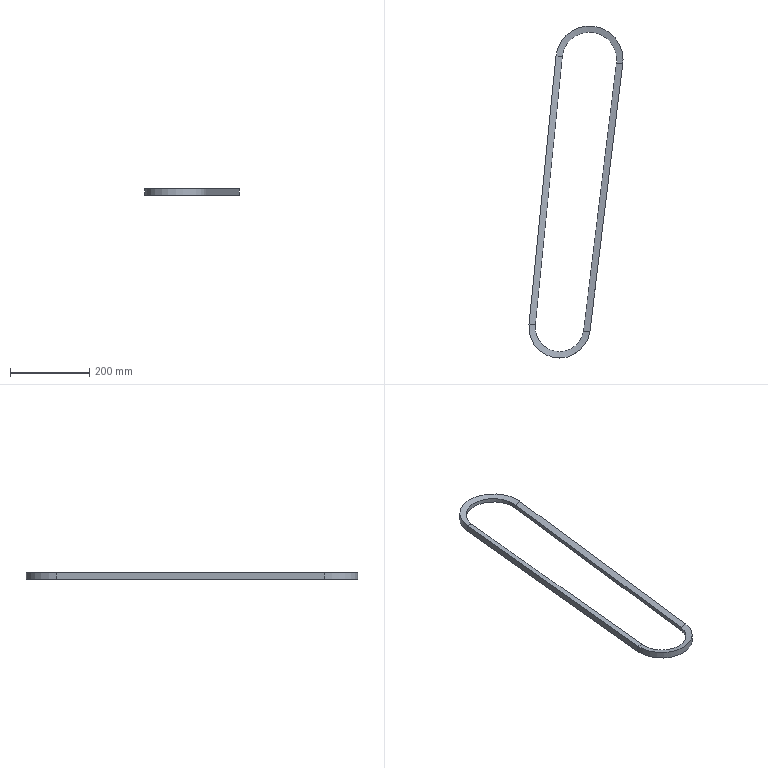Part | SolidWorks | features Sweep 1 | 1 solid | 18 faces | box 238 x 839.181 x 17 mm | volume 391508 mm3 | plane 8 | cylinder 6 | spline 4 | commonest cylinder face diameters 138.293 x2 170 x2 123.3 x1 155 x1
STEP:
#1=CARTESIAN_POINT('',(118.715,333.323,-5.));
#2=VERTEX_POINT('',#1);
#3=CARTESIAN_POINT('',(-19.01,342.17,-5.));
#4=VERTEX_POINT('',#3);
#5=CARTESIAN_POINT('',(49.568,333.323,-5.));
#6=DIRECTION('',(0.,0.,1.));
#7=DIRECTION('',(0.9887,-0.1498,0.));
#8=AXIS2_PLACEMENT_3D('',#5,#6,#7);
#9=CIRCLE('',#8,69.147);
#10=EDGE_CURVE('',#2,#4,#9,.T.);
#11=ORIENTED_EDGE('',*,*,#10,.F.);
#12=CARTESIAN_POINT('',(118.715,333.323,5.));
#13=VERTEX_POINT('',#12);
#14=CARTESIAN_POINT('',(118.715,333.323,0.));
#15=DIRECTION('',(0.,0.,1.));
#16=VECTOR('',#15,1000.);
#17=LINE('',#14,#16);
#18=EDGE_CURVE('',#2,#13,#17,.T.);
#19=ORIENTED_EDGE('',*,*,#18,.T.);
#20=CARTESIAN_POINT('',(-19.01,342.17,5.));
#21=VERTEX_POINT('',#20);
#22=CARTESIAN_POINT('',(49.568,333.323,5.));
#23=DIRECTION('',(0.,0.,1.));
#24=DIRECTION('',(0.9887,-0.1498,0.));
#25=AXIS2_PLACEMENT_3D('',#22,#23,#24);
#26=CIRCLE('',#25,69.147);
#27=EDGE_CURVE('',#13,#21,#26,.T.);
#28=ORIENTED_EDGE('',*,*,#27,.T.);
#29=CARTESIAN_POINT('',(-19.01,342.17,5.));
#30=DIRECTION('',(0.,0.,1.));
#31=VECTOR('',#30,1000.);
#32=LINE('',#29,#31);
#33=EDGE_CURVE('',#4,#21,#32,.T.);
#34=ORIENTED_EDGE('',*,*,#33,.F.);
#35=EDGE_LOOP('',(#11,#19,#28,#34));
#36=FACE_OUTER_BOUND('',#35,.T.);
#37=CARTESIAN_POINT('',(49.568,333.323,0.));
#38=DIRECTION('',(0.,0.,1.));
#39=DIRECTION('',(1.,0.,0.));
#40=AXIS2_PLACEMENT_3D('',#37,#38,#39);
#41=CYLINDRICAL_SURFACE('',#40,69.147);
#42=ADVANCED_FACE('',(#36),#41,.F.);
#43=CARTESIAN_POINT('',(133.935,322.968,-8.5));
#44=VERTEX_POINT('',#43);
#45=CARTESIAN_POINT('',(134.568,333.323,-8.5));
#46=VERTEX_POINT('',#45);
#47=CARTESIAN_POINT('',(49.568,333.323,-8.5));
#48=DIRECTION('',(0.,0.,1.));
#49=DIRECTION('',(0.9926,-0.1218,0.));
#50=AXIS2_PLACEMENT_3D('',#47,#48,#49);
#51=CIRCLE('',#50,85.);
#52=EDGE_CURVE('',#44,#46,#51,.T.);
#53=ORIENTED_EDGE('',*,*,#52,.T.);
#54=CARTESIAN_POINT('',(134.568,333.323,8.5));
#55=VERTEX_POINT('',#54);
#56=CARTESIAN_POINT('',(134.568,333.323,0.));
#57=DIRECTION('',(0.,0.,1.));
#58=VECTOR('',#57,1000.);
#59=LINE('',#56,#58);
#60=EDGE_CURVE('',#46,#55,#59,.T.);
#61=ORIENTED_EDGE('',*,*,#60,.T.);
#62=CARTESIAN_POINT('',(133.935,322.968,8.5));
#63=VERTEX_POINT('',#62);
#64=CARTESIAN_POINT('',(49.568,333.323,8.5));
#65=DIRECTION('',(0.,0.,1.));
#66=DIRECTION('',(0.9926,-0.1218,0.));
#67=AXIS2_PLACEMENT_3D('',#64,#65,#66);
#68=CIRCLE('',#67,85.);
#69=EDGE_CURVE('',#63,#55,#68,.T.);
#70=ORIENTED_EDGE('',*,*,#69,.F.);
#71=CARTESIAN_POINT('',(133.935,322.968,-8.5));
#72=DIRECTION('',(0.,0.,-1.));
#73=VECTOR('',#72,1000.);
#74=LINE('',#71,#73);
#75=EDGE_CURVE('',#63,#44,#74,.T.);
#76=ORIENTED_EDGE('',*,*,#75,.T.);
#77=EDGE_LOOP('',(#53,#61,#70,#76));
#78=FACE_OUTER_BOUND('',#77,.T.);
#79=CARTESIAN_POINT('',(49.568,333.323,0.));
#80=DIRECTION('',(0.,0.,1.));
#81=DIRECTION('',(1.,0.,0.));
#82=AXIS2_PLACEMENT_3D('',#79,#80,#81);
#83=CYLINDRICAL_SURFACE('',#82,85.);
#84=ADVANCED_FACE('',(#78),#83,.T.);
#85=CARTESIAN_POINT('',(50.991,-352.799,8.5));
#86=VERTEX_POINT('',#85);
#87=CARTESIAN_POINT('',(50.991,-352.799,8.5));
#88=DIRECTION('',(0.1218,0.9926,0.));
#89=VECTOR('',#88,1000.);
#90=LINE('',#87,#89);
#91=EDGE_CURVE('',#86,#63,#90,.T.);
#92=ORIENTED_EDGE('',*,*,#91,.F.);
#93=CARTESIAN_POINT('',(50.991,-352.799,-8.5));
#94=VERTEX_POINT('',#93);
#95=CARTESIAN_POINT('',(50.991,-352.799,-8.5));
#96=DIRECTION('',(0.,0.,-1.));
#97=VECTOR('',#96,1000.);
#98=LINE('',#95,#97);
#99=EDGE_CURVE('',#86,#94,#98,.T.);
#100=ORIENTED_EDGE('',*,*,#99,.T.);
#101=CARTESIAN_POINT('',(50.991,-352.799,-8.5));
#102=DIRECTION('',(0.1218,0.9926,0.));
#103=VECTOR('',#102,1000.);
#104=LINE('',#101,#103);
#105=EDGE_CURVE('',#94,#44,#104,.T.);
#106=ORIENTED_EDGE('',*,*,#105,.T.);
#107=ORIENTED_EDGE('',*,*,#75,.F.);
#108=EDGE_LOOP('',(#92,#100,#106,#107));
#109=FACE_OUTER_BOUND('',#108,.T.);
#110=CARTESIAN_POINT('',(50.991,-352.799,-8.5));
#111=DIRECTION('',(0.9926,-0.1218,0.));
#112=DIRECTION('',(0.1218,0.9926,0.));
#113=AXIS2_PLACEMENT_3D('',#110,#111,#112);
#114=PLANE('',#113);
#115=ADVANCED_FACE('',(#109),#114,.T.);
#116=CARTESIAN_POINT('',(34.991,-352.799,5.));
#117=VERTEX_POINT('',#116);
#118=CARTESIAN_POINT('',(117.935,322.968,5.));
#119=VERTEX_POINT('',#118);
#120=CARTESIAN_POINT('',(34.991,-352.799,5.));
#121=DIRECTION('',(0.1218,0.9926,0.));
#122=VECTOR('',#121,1000.);
#123=LINE('',#120,#122);
#124=EDGE_CURVE('',#117,#119,#123,.T.);
#125=ORIENTED_EDGE('',*,*,#124,.F.);
#126=CARTESIAN_POINT('',(50.991,-352.799,8.5));
#127=DIRECTION('',(0.9769,0.,0.2137));
#128=VECTOR('',#127,1000.);
#129=LINE('',#126,#128);
#130=EDGE_CURVE('',#117,#86,#129,.T.);
#131=ORIENTED_EDGE('',*,*,#130,.T.);
#132=ORIENTED_EDGE('',*,*,#91,.T.);
#133=CARTESIAN_POINT('',(133.935,322.968,8.5));
#134=DIRECTION('',(0.9769,0.,0.2137));
#135=VECTOR('',#134,1000.);
#136=LINE('',#133,#135);
#137=EDGE_CURVE('',#119,#63,#136,.T.);
#138=ORIENTED_EDGE('',*,*,#137,.F.);
#139=EDGE_LOOP('',(#125,#131,#132,#138));
#140=FACE_OUTER_BOUND('',#139,.T.);
#141=CARTESIAN_POINT('',(50.991,-352.799,8.5));
#142=DIRECTION('',(-0.2136,0.02622,0.9766));
#143=DIRECTION('',(0.9769,0.,0.2137));
#144=AXIS2_PLACEMENT_3D('',#141,#142,#143);
#145=PLANE('',#144);
#146=ADVANCED_FACE('',(#140),#145,.T.);
#147=CARTESIAN_POINT('',(34.991,-352.799,-5.));
#148=VERTEX_POINT('',#147);
#149=CARTESIAN_POINT('',(117.935,322.968,-5.));
#150=VERTEX_POINT('',#149);
#151=CARTESIAN_POINT('',(34.991,-352.799,-5.));
#152=DIRECTION('',(0.1218,0.9926,0.));
#153=VECTOR('',#152,1000.);
#154=LINE('',#151,#153);
#155=EDGE_CURVE('',#148,#150,#154,.T.);
#156=ORIENTED_EDGE('',*,*,#155,.F.);
#157=CARTESIAN_POINT('',(34.991,-352.799,5.));
#158=DIRECTION('',(0.,0.,1.));
#159=VECTOR('',#158,1000.);
#160=LINE('',#157,#159);
#161=EDGE_CURVE('',#148,#117,#160,.T.);
#162=ORIENTED_EDGE('',*,*,#161,.T.);
#163=ORIENTED_EDGE('',*,*,#124,.T.);
#164=CARTESIAN_POINT('',(117.935,322.968,5.));
#165=DIRECTION('',(0.,0.,1.));
#166=VECTOR('',#165,1000.);
#167=LINE('',#164,#166);
#168=EDGE_CURVE('',#150,#119,#167,.T.);
#169=ORIENTED_EDGE('',*,*,#168,.F.);
#170=EDGE_LOOP('',(#156,#162,#163,#169));
#171=FACE_OUTER_BOUND('',#170,.T.);
#172=CARTESIAN_POINT('',(34.991,-352.799,5.));
#173=DIRECTION('',(-0.9926,0.1218,0.));
#174=DIRECTION('',(-0.1218,-0.9926,0.));
#175=AXIS2_PLACEMENT_3D('',#172,#173,#174);
#176=PLANE('',#175);
#177=ADVANCED_FACE('',(#171),#176,.T.);
#178=ORIENTED_EDGE('',*,*,#99,.F.);
#179=CARTESIAN_POINT('',(-103.044,-335.613,8.5));
#180=VERTEX_POINT('',#179);
#181=CARTESIAN_POINT('',(-25.932,-343.358,8.5));
#182=DIRECTION('',(0.,0.,1.));
#183=DIRECTION('',(-0.995,0.09993,0.));
#184=AXIS2_PLACEMENT_3D('',#181,#182,#183);
#185=CIRCLE('',#184,77.5);
#186=EDGE_CURVE('',#180,#86,#185,.T.);
#187=ORIENTED_EDGE('',*,*,#186,.F.);
#188=CARTESIAN_POINT('',(-103.044,-335.613,-8.5));
#189=VERTEX_POINT('',#188);
#190=CARTESIAN_POINT('',(-103.044,-335.613,-8.5));
#191=DIRECTION('',(0.,0.,-1.));
#192=VECTOR('',#191,1000.);
#193=LINE('',#190,#192);
#194=EDGE_CURVE('',#180,#189,#193,.T.);
#195=ORIENTED_EDGE('',*,*,#194,.T.);
#196=CARTESIAN_POINT('',(-25.932,-343.358,-8.5));
#197=DIRECTION('',(0.,0.,1.));
#198=DIRECTION('',(-0.995,0.09993,0.));
#199=AXIS2_PLACEMENT_3D('',#196,#197,#198);
#200=CIRCLE('',#199,77.5);
#201=EDGE_CURVE('',#189,#94,#200,.T.);
#202=ORIENTED_EDGE('',*,*,#201,.T.);
#203=EDGE_LOOP('',(#178,#187,#195,#202));
#204=FACE_OUTER_BOUND('',#203,.T.);
#205=CARTESIAN_POINT('',(-25.932,-343.358,0.));
#206=DIRECTION('',(0.,0.,1.));
#207=DIRECTION('',(1.,0.,0.));
#208=AXIS2_PLACEMENT_3D('',#205,#206,#207);
#209=CYLINDRICAL_SURFACE('',#208,77.5);
#210=ADVANCED_FACE('',(#204),#209,.T.);
#211=ORIENTED_EDGE('',*,*,#186,.T.);
#212=ORIENTED_EDGE('',*,*,#130,.F.);
#213=CARTESIAN_POINT('',(-87.048,-335.261,5.));
#214=VERTEX_POINT('',#213);
#215=CARTESIAN_POINT('',(-25.932,-343.358,5.));
#216=DIRECTION('',(0.,0.,1.));
#217=DIRECTION('',(-0.9913,0.1313,0.));
#218=AXIS2_PLACEMENT_3D('',#215,#216,#217);
#219=CIRCLE('',#218,61.65);
#220=EDGE_CURVE('',#214,#117,#219,.T.);
#221=ORIENTED_EDGE('',*,*,#220,.F.);
#222=CARTESIAN_POINT('',(-103.044,-335.613,8.5));
#223=DIRECTION('',(-0.9767,-0.02152,0.2137));
#224=VECTOR('',#223,1000.);
#225=LINE('',#222,#224);
#226=EDGE_CURVE('',#214,#180,#225,.T.);
#227=ORIENTED_EDGE('',*,*,#226,.T.);
#228=EDGE_LOOP('',(#211,#212,#221,#227));
#229=FACE_OUTER_BOUND('',#228,.T.);
#230=CARTESIAN_POINT('',(-87.048,-335.261,5.));
#231=CARTESIAN_POINT('',(-102.892,-454.851,5.));
#232=CARTESIAN_POINT('',(16.516,-472.011,5.));
#233=CARTESIAN_POINT('',(34.991,-352.799,5.));
#234=CARTESIAN_POINT('',(-103.044,-335.613,8.5));
#235=CARTESIAN_POINT('',(-118.199,-486.504,8.5));
#236=CARTESIAN_POINT('',(32.516,-503.32,8.5));
#237=CARTESIAN_POINT('',(50.991,-352.799,8.5));
#238=(BOUNDED_SURFACE()B_SPLINE_SURFACE(1,3,((#230,#231,#232,#233),(#234,#235,#236,#237)),.UNSPECIFIED.,.F.,.F.,.F.)B_SPLINE_SURFACE_WITH_KNOTS((2,2),(4,4),(0.,1.),(0.,1.),.UNSPECIFIED.)GEOMETRIC_REPRESENTATION_ITEM()RATIONAL_B_SPLINE_SURFACE(((1.,0.3407,0.3407,1.),(1.,0.3407,0.3407,1.)))REPRESENTATION_ITEM('')SURFACE());
#239=ADVANCED_FACE('',(#229),#238,.T.);
#240=ORIENTED_EDGE('',*,*,#220,.T.);
#241=ORIENTED_EDGE('',*,*,#161,.F.);
#242=CARTESIAN_POINT('',(-87.048,-335.261,-5.));
#243=VERTEX_POINT('',#242);
#244=CARTESIAN_POINT('',(-25.932,-343.358,-5.));
#245=DIRECTION('',(0.,0.,1.));
#246=DIRECTION('',(-0.9913,0.1313,0.));
#247=AXIS2_PLACEMENT_3D('',#244,#245,#246);
#248=CIRCLE('',#247,61.65);
#249=EDGE_CURVE('',#243,#148,#248,.T.);
#250=ORIENTED_EDGE('',*,*,#249,.F.);
#251=CARTESIAN_POINT('',(-87.048,-335.261,5.));
#252=DIRECTION('',(0.,0.,1.));
#253=VECTOR('',#252,1000.);
#254=LINE('',#251,#253);
#255=EDGE_CURVE('',#243,#214,#254,.T.);
#256=ORIENTED_EDGE('',*,*,#255,.T.);
#257=EDGE_LOOP('',(#240,#241,#250,#256));
#258=FACE_OUTER_BOUND('',#257,.T.);
#259=CARTESIAN_POINT('',(-25.932,-343.358,0.));
#260=DIRECTION('',(0.,0.,1.));
#261=DIRECTION('',(1.,0.,0.));
#262=AXIS2_PLACEMENT_3D('',#259,#260,#261);
#263=CYLINDRICAL_SURFACE('',#262,61.65);
#264=ADVANCED_FACE('',(#258),#263,.F.);
#265=ORIENTED_EDGE('',*,*,#249,.T.);
#266=CARTESIAN_POINT('',(50.991,-352.799,-8.5));
#267=DIRECTION('',(-0.9769,0.,0.2137));
#268=VECTOR('',#267,1000.);
#269=LINE('',#266,#268);
#270=EDGE_CURVE('',#94,#148,#269,.T.);
#271=ORIENTED_EDGE('',*,*,#270,.F.);
#272=ORIENTED_EDGE('',*,*,#201,.F.);
#273=CARTESIAN_POINT('',(-103.044,-335.613,-8.5));
#274=DIRECTION('',(0.9767,0.02152,0.2137));
#275=VECTOR('',#274,1000.);
#276=LINE('',#273,#275);
#277=EDGE_CURVE('',#189,#243,#276,.T.);
#278=ORIENTED_EDGE('',*,*,#277,.T.);
#279=EDGE_LOOP('',(#265,#271,#272,#278));
#280=FACE_OUTER_BOUND('',#279,.T.);
#281=CARTESIAN_POINT('',(-103.044,-335.613,-8.5));
#282=CARTESIAN_POINT('',(-118.199,-486.504,-8.5));
#283=CARTESIAN_POINT('',(32.516,-503.32,-8.5));
#284=CARTESIAN_POINT('',(50.991,-352.799,-8.5));
#285=CARTESIAN_POINT('',(-87.048,-335.261,-5.));
#286=CARTESIAN_POINT('',(-102.892,-454.851,-5.));
#287=CARTESIAN_POINT('',(16.516,-472.011,-5.));
#288=CARTESIAN_POINT('',(34.991,-352.799,-5.));
#289=(BOUNDED_SURFACE()B_SPLINE_SURFACE(1,3,((#281,#282,#283,#284),(#285,#286,#287,#288)),.UNSPECIFIED.,.F.,.F.,.F.)B_SPLINE_SURFACE_WITH_KNOTS((2,2),(4,4),(0.,1.),(0.,1.),.UNSPECIFIED.)GEOMETRIC_REPRESENTATION_ITEM()RATIONAL_B_SPLINE_SURFACE(((1.,0.3407,0.3407,1.),(1.,0.3407,0.3407,1.)))REPRESENTATION_ITEM('')SURFACE());
#290=ADVANCED_FACE('',(#280),#289,.T.);
#291=ORIENTED_EDGE('',*,*,#194,.F.);
#292=CARTESIAN_POINT('',(-35.006,341.818,8.5));
#293=VERTEX_POINT('',#292);
#294=CARTESIAN_POINT('',(-35.006,341.818,8.5));
#295=DIRECTION('',(-0.09993,-0.995,0.));
#296=VECTOR('',#295,1000.);
#297=LINE('',#294,#296);
#298=EDGE_CURVE('',#293,#180,#297,.T.);
#299=ORIENTED_EDGE('',*,*,#298,.F.);
#300=CARTESIAN_POINT('',(-35.006,341.818,-8.5));
#301=VERTEX_POINT('',#300);
#302=CARTESIAN_POINT('',(-35.006,341.818,-8.5));
#303=DIRECTION('',(0.,0.,-1.));
#304=VECTOR('',#303,1000.);
#305=LINE('',#302,#304);
#306=EDGE_CURVE('',#293,#301,#305,.T.);
#307=ORIENTED_EDGE('',*,*,#306,.T.);
#308=CARTESIAN_POINT('',(-35.006,341.818,-8.5));
#309=DIRECTION('',(-0.09993,-0.995,0.));
#310=VECTOR('',#309,1000.);
#311=LINE('',#308,#310);
#312=EDGE_CURVE('',#301,#189,#311,.T.);
#313=ORIENTED_EDGE('',*,*,#312,.T.);
#314=EDGE_LOOP('',(#291,#299,#307,#313));
#315=FACE_OUTER_BOUND('',#314,.T.);
#316=CARTESIAN_POINT('',(-35.006,341.818,-8.5));
#317=DIRECTION('',(-0.995,0.09993,0.));
#318=DIRECTION('',(-0.09993,-0.995,0.));
#319=AXIS2_PLACEMENT_3D('',#316,#317,#318);
#320=PLANE('',#319);
#321=ADVANCED_FACE('',(#315),#320,.T.);
#322=ORIENTED_EDGE('',*,*,#298,.T.);
#323=ORIENTED_EDGE('',*,*,#226,.F.);
#324=CARTESIAN_POINT('',(-19.01,342.17,5.));
#325=DIRECTION('',(-0.09993,-0.995,0.));
#326=VECTOR('',#325,1000.);
#327=LINE('',#324,#326);
#328=EDGE_CURVE('',#21,#214,#327,.T.);
#329=ORIENTED_EDGE('',*,*,#328,.F.);
#330=CARTESIAN_POINT('',(-35.006,341.818,8.5));
#331=DIRECTION('',(-0.9767,-0.02152,0.2137));
#332=VECTOR('',#331,1000.);
#333=LINE('',#330,#332);
#334=EDGE_CURVE('',#21,#293,#333,.T.);
#335=ORIENTED_EDGE('',*,*,#334,.T.);
#336=EDGE_LOOP('',(#322,#323,#329,#335));
#337=FACE_OUTER_BOUND('',#336,.T.);
#338=CARTESIAN_POINT('',(-35.006,341.818,8.5));
#339=DIRECTION('',(0.2141,-0.02151,0.9766));
#340=DIRECTION('',(0.9768,0.,-0.2142));
#341=AXIS2_PLACEMENT_3D('',#338,#339,#340);
#342=PLANE('',#341);
#343=ADVANCED_FACE('',(#337),#342,.T.);
#344=ORIENTED_EDGE('',*,*,#328,.T.);
#345=ORIENTED_EDGE('',*,*,#255,.F.);
#346=CARTESIAN_POINT('',(-19.01,342.17,-5.));
#347=DIRECTION('',(-0.09993,-0.995,0.));
#348=VECTOR('',#347,1000.);
#349=LINE('',#346,#348);
#350=EDGE_CURVE('',#4,#243,#349,.T.);
#351=ORIENTED_EDGE('',*,*,#350,.F.);
#352=ORIENTED_EDGE('',*,*,#33,.T.);
#353=EDGE_LOOP('',(#344,#345,#351,#352));
#354=FACE_OUTER_BOUND('',#353,.T.);
#355=CARTESIAN_POINT('',(-19.01,342.17,5.));
#356=DIRECTION('',(0.995,-0.09993,0.));
#357=DIRECTION('',(0.09993,0.995,0.));
#358=AXIS2_PLACEMENT_3D('',#355,#356,#357);
#359=PLANE('',#358);
#360=ADVANCED_FACE('',(#354),#359,.T.);
#361=ORIENTED_EDGE('',*,*,#350,.T.);
#362=ORIENTED_EDGE('',*,*,#277,.F.);
#363=ORIENTED_EDGE('',*,*,#312,.F.);
#364=CARTESIAN_POINT('',(-35.006,341.818,-8.5));
#365=DIRECTION('',(0.9767,0.02152,0.2137));
#366=VECTOR('',#365,1000.);
#367=LINE('',#364,#366);
#368=EDGE_CURVE('',#301,#4,#367,.T.);
#369=ORIENTED_EDGE('',*,*,#368,.T.);
#370=EDGE_LOOP('',(#361,#362,#363,#369));
#371=FACE_OUTER_BOUND('',#370,.T.);
#372=CARTESIAN_POINT('',(-35.006,341.818,-8.5));
#373=DIRECTION('',(0.2141,-0.02151,-0.9766));
#374=DIRECTION('',(-0.9768,0.,-0.2142));
#375=AXIS2_PLACEMENT_3D('',#372,#373,#374);
#376=PLANE('',#375);
#377=ADVANCED_FACE('',(#371),#376,.T.);
#378=ORIENTED_EDGE('',*,*,#60,.F.);
#379=CARTESIAN_POINT('',(49.568,333.323,-8.5));
#380=DIRECTION('',(0.,0.,1.));
#381=DIRECTION('',(0.9926,-0.1218,0.));
#382=AXIS2_PLACEMENT_3D('',#379,#380,#381);
#383=CIRCLE('',#382,85.);
#384=EDGE_CURVE('',#46,#301,#383,.T.);
#385=ORIENTED_EDGE('',*,*,#384,.T.);
#386=ORIENTED_EDGE('',*,*,#306,.F.);
#387=CARTESIAN_POINT('',(49.568,333.323,8.5));
#388=DIRECTION('',(0.,0.,1.));
#389=DIRECTION('',(0.9926,-0.1218,0.));
#390=AXIS2_PLACEMENT_3D('',#387,#388,#389);
#391=CIRCLE('',#390,85.);
#392=EDGE_CURVE('',#55,#293,#391,.T.);
#393=ORIENTED_EDGE('',*,*,#392,.F.);
#394=EDGE_LOOP('',(#378,#385,#386,#393));
#395=FACE_OUTER_BOUND('',#394,.T.);
#396=CARTESIAN_POINT('',(49.568,333.323,0.));
#397=DIRECTION('',(0.,0.,1.));
#398=DIRECTION('',(1.,0.,0.));
#399=AXIS2_PLACEMENT_3D('',#396,#397,#398);
#400=CYLINDRICAL_SURFACE('',#399,85.);
#401=ADVANCED_FACE('',(#395),#400,.T.);
#402=ORIENTED_EDGE('',*,*,#69,.T.);
#403=ORIENTED_EDGE('',*,*,#392,.T.);
#404=ORIENTED_EDGE('',*,*,#334,.F.);
#405=ORIENTED_EDGE('',*,*,#27,.F.);
#406=CARTESIAN_POINT('',(49.568,333.323,5.));
#407=DIRECTION('',(0.,0.,1.));
#408=DIRECTION('',(0.9887,-0.1498,0.));
#409=AXIS2_PLACEMENT_3D('',#406,#407,#408);
#410=CIRCLE('',#409,69.147);
#411=EDGE_CURVE('',#119,#13,#410,.T.);
#412=ORIENTED_EDGE('',*,*,#411,.F.);
#413=ORIENTED_EDGE('',*,*,#137,.T.);
#414=EDGE_LOOP('',(#402,#403,#404,#405,#412,#413));
#415=FACE_OUTER_BOUND('',#414,.T.);
#416=CARTESIAN_POINT('',(117.935,322.968,5.));
#417=CARTESIAN_POINT('',(124.054,363.367,5.));
#418=CARTESIAN_POINT('',(99.634,396.127,5.));
#419=CARTESIAN_POINT('',(59.17,401.8,5.));
#420=CARTESIAN_POINT('',(18.706,407.474,5.));
#421=CARTESIAN_POINT('',(-13.783,382.694,5.));
#422=CARTESIAN_POINT('',(-19.01,342.17,5.));
#423=CARTESIAN_POINT('',(133.935,322.968,8.5));
#424=CARTESIAN_POINT('',(140.054,372.822,8.5));
#425=CARTESIAN_POINT('',(108.912,412.23,8.5));
#426=CARTESIAN_POINT('',(58.993,417.799,8.5));
#427=CARTESIAN_POINT('',(9.075,423.369,8.5));
#428=CARTESIAN_POINT('',(-29.987,391.794,8.5));
#429=CARTESIAN_POINT('',(-35.006,341.818,8.5));
#430=(BOUNDED_SURFACE()B_SPLINE_SURFACE(1,3,((#416,#417,#418,#419,#420,#421,#422),(#423,#424,#425,#426,#427,#428,#429)),.UNSPECIFIED.,.F.,.F.,.F.)B_SPLINE_SURFACE_WITH_KNOTS((2,2),(4,3,4),(0.,1.),(0.,0.5,1.),.UNSPECIFIED.)GEOMETRIC_REPRESENTATION_ITEM()RATIONAL_B_SPLINE_SURFACE(((1.,0.8021,0.8021,1.,0.8021,0.8021,1.),(1.,0.8021,0.8021,1.,0.8021,0.8021,1.)))REPRESENTATION_ITEM('')SURFACE());
#431=ADVANCED_FACE('',(#415),#430,.T.);
#432=ORIENTED_EDGE('',*,*,#18,.F.);
#433=CARTESIAN_POINT('',(49.568,333.323,-5.));
#434=DIRECTION('',(0.,0.,1.));
#435=DIRECTION('',(0.9887,-0.1498,0.));
#436=AXIS2_PLACEMENT_3D('',#433,#434,#435);
#437=CIRCLE('',#436,69.147);
#438=EDGE_CURVE('',#150,#2,#437,.T.);
#439=ORIENTED_EDGE('',*,*,#438,.F.);
#440=ORIENTED_EDGE('',*,*,#168,.T.);
#441=ORIENTED_EDGE('',*,*,#411,.T.);
#442=EDGE_LOOP('',(#432,#439,#440,#441));
#443=FACE_OUTER_BOUND('',#442,.T.);
#444=CARTESIAN_POINT('',(49.568,333.323,0.));
#445=DIRECTION('',(0.,0.,1.));
#446=DIRECTION('',(1.,0.,0.));
#447=AXIS2_PLACEMENT_3D('',#444,#445,#446);
#448=CYLINDRICAL_SURFACE('',#447,69.147);
#449=ADVANCED_FACE('',(#443),#448,.F.);
#450=ORIENTED_EDGE('',*,*,#438,.T.);
#451=ORIENTED_EDGE('',*,*,#10,.T.);
#452=ORIENTED_EDGE('',*,*,#368,.F.);
#453=ORIENTED_EDGE('',*,*,#384,.F.);
#454=ORIENTED_EDGE('',*,*,#52,.F.);
#455=CARTESIAN_POINT('',(133.935,322.968,-8.5));
#456=DIRECTION('',(-0.9769,0.,0.2137));
#457=VECTOR('',#456,1000.);
#458=LINE('',#455,#457);
#459=EDGE_CURVE('',#44,#150,#458,.T.);
#460=ORIENTED_EDGE('',*,*,#459,.T.);
#461=EDGE_LOOP('',(#450,#451,#452,#453,#454,#460));
#462=FACE_OUTER_BOUND('',#461,.T.);
#463=CARTESIAN_POINT('',(133.935,322.968,-8.5));
#464=CARTESIAN_POINT('',(140.054,372.822,-8.5));
#465=CARTESIAN_POINT('',(108.912,412.23,-8.5));
#466=CARTESIAN_POINT('',(58.993,417.799,-8.5));
#467=CARTESIAN_POINT('',(9.075,423.369,-8.5));
#468=CARTESIAN_POINT('',(-29.987,391.794,-8.5));
#469=CARTESIAN_POINT('',(-35.006,341.818,-8.5));
#470=CARTESIAN_POINT('',(117.935,322.968,-5.));
#471=CARTESIAN_POINT('',(124.054,363.367,-5.));
#472=CARTESIAN_POINT('',(99.634,396.127,-5.));
#473=CARTESIAN_POINT('',(59.17,401.8,-5.));
#474=CARTESIAN_POINT('',(18.706,407.474,-5.));
#475=CARTESIAN_POINT('',(-13.783,382.694,-5.));
#476=CARTESIAN_POINT('',(-19.01,342.17,-5.));
#477=(BOUNDED_SURFACE()B_SPLINE_SURFACE(1,3,((#463,#464,#465,#466,#467,#468,#469),(#470,#471,#472,#473,#474,#475,#476)),.UNSPECIFIED.,.F.,.F.,.F.)B_SPLINE_SURFACE_WITH_KNOTS((2,2),(4,3,4),(0.,1.),(0.,0.5,1.),.UNSPECIFIED.)GEOMETRIC_REPRESENTATION_ITEM()RATIONAL_B_SPLINE_SURFACE(((1.,0.8021,0.8021,1.,0.8021,0.8021,1.),(1.,0.8021,0.8021,1.,0.8021,0.8021,1.)))REPRESENTATION_ITEM('')SURFACE());
#478=ADVANCED_FACE('',(#462),#477,.T.);
#479=ORIENTED_EDGE('',*,*,#270,.T.);
#480=ORIENTED_EDGE('',*,*,#155,.T.);
#481=ORIENTED_EDGE('',*,*,#459,.F.);
#482=ORIENTED_EDGE('',*,*,#105,.F.);
#483=EDGE_LOOP('',(#479,#480,#481,#482));
#484=FACE_OUTER_BOUND('',#483,.T.);
#485=CARTESIAN_POINT('',(50.991,-352.799,-8.5));
#486=DIRECTION('',(-0.2136,0.02622,-0.9766));
#487=DIRECTION('',(-0.9769,0.,0.2137));
#488=AXIS2_PLACEMENT_3D('',#485,#486,#487);
#489=PLANE('',#488);
#490=ADVANCED_FACE('',(#484),#489,.T.);
#491=CLOSED_SHELL('',(#42,#84,#115,#146,#177,#210,#239,#264,#290,#321,#343,#360,#377,#401,#431,#449,#478,#490));
#492=MANIFOLD_SOLID_BREP('',#491);
#493=CARTESIAN_POINT('',(0.,0.,0.));
#494=DIRECTION('',(0.,0.,1.));
#495=DIRECTION('',(1.,0.,0.));
#496=AXIS2_PLACEMENT_3D('',#493,#494,#495);
#497=(LENGTH_UNIT()NAMED_UNIT(*)SI_UNIT(.MILLI.,.METRE.));
#498=UNCERTAINTY_MEASURE_WITH_UNIT(LENGTH_MEASURE(0.00001),#497,'','');
#499=(NAMED_UNIT(*)PLANE_ANGLE_UNIT()SI_UNIT($,.RADIAN.));
#500=(NAMED_UNIT(*)SI_UNIT($,.STERADIAN.)SOLID_ANGLE_UNIT());
#501=(GEOMETRIC_REPRESENTATION_CONTEXT(3)GLOBAL_UNCERTAINTY_ASSIGNED_CONTEXT((#498))GLOBAL_UNIT_ASSIGNED_CONTEXT((#497,#499,#500))REPRESENTATION_CONTEXT('',''));
#502=ADVANCED_BREP_SHAPE_REPRESENTATION('',(#492,#496),#501);